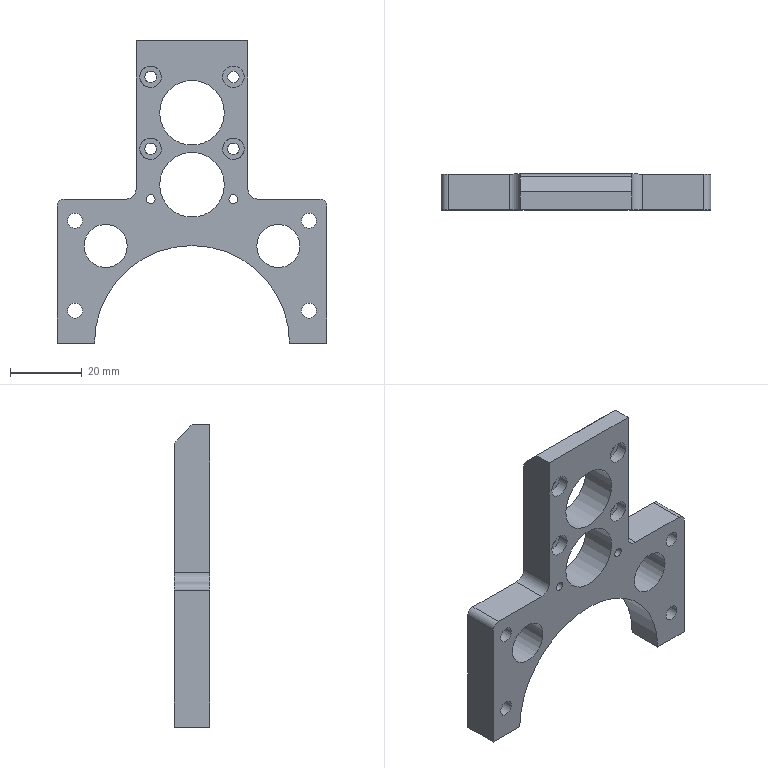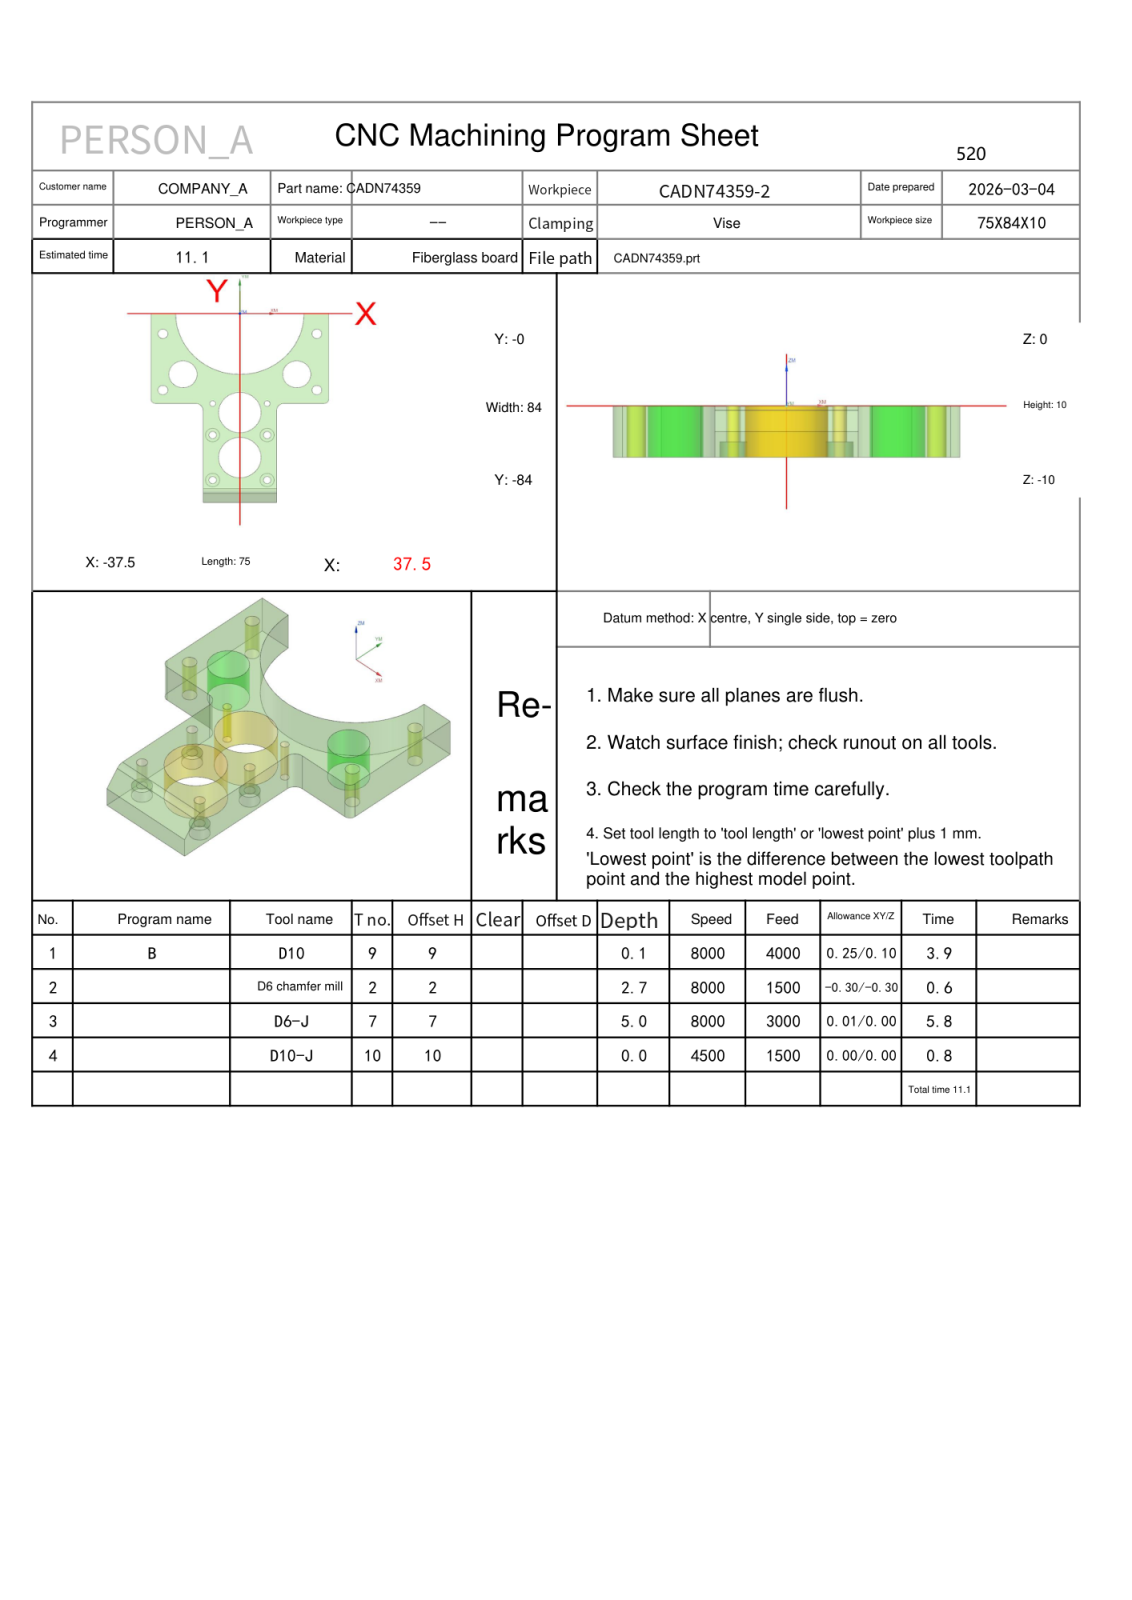NC program | NX | posted by the shop | part box 75 x 10 x 84 mm
Lines 1701 to 1963 of 5701:
N2 T02 M06
(D6 chamfer mill  D=6. R=0. H=02 ce=0.00 di=0.10)
G00 G90 G54 X-11.5 Y-40. M03 S8000
G43 H02 Z50.
M08
G98 G81 X-11.5 Y-40. Z-1.75 R3. F1000.
X11.5
G80
G00 Z50.
G00 G90 X-11.5 Y-74. M03 S8000
Z50.
G98 G81 X-11.5 Y-74. Z-1.9 R3. F1000.
Y-54.
X11.5
Y-74.
G80
G00 Z50.
G00 G90 X32.5 Y-34. M03 S8000
Z50.
G98 G81 X32.5 Y-34. Z-2.7 R3. F1000.
Y-9.
X-32.5
Y-34.
G80
G00 Z50.
G00 G90 X-21. Y-24.7 M03 S8000
Z50.
Z-.5
G01 Z-1. F1200.
G03 X-24. Y-21.7 I-3. J0.0
X-29.3 Y-27. I0.0 J-5.3
X-24. Y-32.3 I5.3 J0.0
X-18.7 Y-27. I0.0 J5.3
X-24. Y-21.7 I-5.3 J0.0
X-27. Y-24.7 I0.0 J-3.
G01 Z-.5
G00 Z50.
X27.
Z-.5
G01 Z-1.
G03 X24. Y-21.7 I-3. J0.0
X18.7 Y-27. I0.0 J-5.3
X24. Y-32.3 I5.3 J0.0
X29.3 Y-27. I0.0 J5.3
X24. Y-21.7 I-5.3 J0.0
X21. Y-24.7 I0.0 J-3.
G01 Z-.5
G00 Z50.
G00 G90 X-16.727 Y-78.143 M03 S6500
Z50.
Z.145
G01 Z-1.2 F1500.
G03 X-16.527 Y-77.857 I-1.532 J1.286
G01 X-16.497 Y-77.812
X-16.5 Y-77.757
Y-43.
G03 X-18.5 Y-41. I-2. J0.0
G01 X-35.5
G02 X-38.5 Y-38. I0.0 J3.
G01 Y0.0
G02 X-37.5 Y1. I1. J0.0
G01 X-27.1
G02 X-26.1 Y0.0 I0.0 J-1.
G03 X0.0 Y-26.1 I26.1 J0.0
X26.1 Y0.0 I0.0 J26.1
G02 X27.1 Y1. I1. J0.0
G01 X37.5
G02 X38.5 Y0.0 I0.0 J-1.
G01 Y-38.
G02 X35.5 Y-41. I-3. J0.0
G01 X18.5
G03 X16.5 Y-43. I0.0 J-2.
G01 Y-77.757
X16.497 Y-77.812
X16.527 Y-77.857
G03 X16.727 Y-78.143 I1.732 J1.
G01 Z.145
G00 Z2.55
X11.919 Y-73.556
Z.417
G01 Z-1.2
G03 X11.603 Y-73.409 I-1. J-1.732
G01 X11.553 Y-73.388
X11.5 Y-73.4
G03 X10.9 Y-74. I0.0 J-.6
X11.5 Y-74.6 I.6 J0.0
X12.1 Y-74. I0.0 J.6
X11.5 Y-73.4 I-.6 J0.0
G01 X11.447 Y-73.388
X11.397 Y-73.409
G03 X11.081 Y-73.556 I.684 J-1.879
G01 Z.417
G00 Z10.
X.396 Y-56.208
Z.209
G01 Z-1.2
G03 X.101 Y-56.022 I-1.211 J-1.592
G01 X.054 Y-55.995
X0.0 Y-56.
G03 X-8. Y-64. I0.0 J-8.
X0.0 Y-72. I8. J0.0
X8. Y-64. I0.0 J8.
X0.0 Y-56. I-8. J0.0
G01 X-.054 Y-55.995
X-.101 Y-56.022
G03 X-.396 Y-56.208 I.916 J-1.778
G01 Z.208
G00 Z10.
X-11.919 Y-74.444
Z.417
G01 Z-1.2
G03 X-11.603 Y-74.591 I1. J1.732
G01 X-11.553 Y-74.612
X-11.5 Y-74.6
G03 X-10.9 Y-74. I0.0 J.6
X-11.5 Y-73.4 I-.6 J0.0
X-12.1 Y-74. I0.0 J-.6
X-11.5 Y-74.6 I.6 J0.0
G01 X-11.447 Y-74.612
X-11.397 Y-74.591
G03 X-11.081 Y-74.444 I-.684 J1.879
G01 Z.417
G00 Z10.
X-11.919 Y-54.444
Z.417
G01 Z-1.2
G03 X-11.603 Y-54.591 I1. J1.732
G01 X-11.553 Y-54.612
X-11.5 Y-54.6
G03 X-10.9 Y-54. I0.0 J.6
X-11.5 Y-53.4 I-.6 J0.0
X-12.1 Y-54. I0.0 J-.6
X-11.5 Y-54.6 I.6 J0.0
G01 X-11.447 Y-54.612
X-11.397 Y-54.591
G03 X-11.081 Y-54.444 I-.684 J1.879
G01 Z.417
G00 Z10.
X-32.912 Y-34.926
Z.321
G01 Z-1.2
G03 X-32.603 Y-35.086 I1.075 J1.687
G01 X-32.554 Y-35.11
X-32.5 Y-35.1
G03 X-31.4 Y-34. I0.0 J1.1
X-32.5 Y-32.9 I-1.1 J0.0
X-33.6 Y-34. I0.0 J-1.1
X-32.5 Y-35.1 I1.1 J0.0
G01 X-32.446 Y-35.11
X-32.397 Y-35.086
G03 X-32.088 Y-34.926 I-.765 J1.848
G01 Z.317
G00 Z10.
X-32.912 Y-9.926
Z.321
G01 Z-1.2
G03 X-32.603 Y-10.086 I1.075 J1.687
G01 X-32.554 Y-10.11
X-32.5 Y-10.1
G03 X-31.4 Y-9. I0.0 J1.1
X-32.5 Y-7.9 I-1.1 J0.0
X-33.6 Y-9. I0.0 J-1.1
X-32.5 Y-10.1 I1.1 J0.0
G01 X-32.446 Y-10.11
X-32.397 Y-10.086
G03 X-32.088 Y-9.926 I-.765 J1.848
G01 Z.317
G00 Z10.
X-23.602 Y-22.204
Z.221
G01 Z-1.2
G03 X-23.899 Y-22.021 I-1.194 J-1.604
G01 X-23.946 Y-21.994
X-24. Y-22.
G03 X-29. Y-27. I0.0 J-5.
X-24. Y-32. I5. J0.0
X-19. Y-27. I0.0 J5.
X-24. Y-22. I-5. J0.0
G01 X-24.054 Y-21.994
X-24.101 Y-22.021
G03 X-24.398 Y-22.204 I.898 J-1.787
G01 Z.214
G00 Z10.
X.396 Y-36.208
Z.209
G01 Z-1.2
G03 X.101 Y-36.022 I-1.211 J-1.592
G01 X.054 Y-35.995
X0.0 Y-36.
G03 X-8. Y-44. I0.0 J-8.
X0.0 Y-52. I8. J0.0
X8. Y-44. I0.0 J8.
X0.0 Y-36. I-8. J0.0
G01 X-.054 Y-35.995
X-.101 Y-36.022
G03 X-.396 Y-36.208 I.916 J-1.778
G01 Z.208
G00 Z10.
X11.919 Y-53.556
Z.417
G01 Z-1.2
G03 X11.603 Y-53.409 I-1. J-1.732
G01 X11.553 Y-53.388
X11.5 Y-53.4
G03 X10.9 Y-54. I0.0 J-.6
X11.5 Y-54.6 I.6 J0.0
X12.1 Y-54. I0.0 J.6
X11.5 Y-53.4 I-.6 J0.0
G01 X11.447 Y-53.388
X11.397 Y-53.409
G03 X11.081 Y-53.556 I.684 J-1.879
G01 Z.417
G00 Z10.
X32.088 Y-34.926
Z.321
G01 Z-1.2
G03 X32.397 Y-35.086 I1.075 J1.687
G01 X32.446 Y-35.11
X32.5 Y-35.1
G03 X33.6 Y-34. I0.0 J1.1
X32.5 Y-32.9 I-1.1 J0.0
X31.4 Y-34. I0.0 J-1.1
X32.5 Y-35.1 I1.1 J0.0
G01 X32.554 Y-35.11
X32.603 Y-35.086
G03 X32.912 Y-34.926 I-.765 J1.848
G01 Z.317
G00 Z10.
X24.398 Y-22.204
Z.221
G01 Z-1.2
G03 X24.101 Y-22.021 I-1.194 J-1.604
G01 X24.054 Y-21.994
X24. Y-22.
G03 X19. Y-27. I0.0 J-5.
X24. Y-32. I5. J0.0
X29. Y-27. I0.0 J5.
X24. Y-22. I-5. J0.0
G01 X23.946 Y-21.994
X23.899 Y-22.021
G03 X23.602 Y-22.204 I.898 J-1.787
G01 Z.214
G00 Z10.
X32.088 Y-9.926
Z.321
G01 Z-1.2
G03 X32.397 Y-10.086 I1.075 J1.687
G01 X32.446 Y-10.11
X32.5 Y-10.1
G03 X33.6 Y-9. I0.0 J1.1
X32.5 Y-7.9 I-1.1 J0.0
X31.4 Y-9. I0.0 J-1.1
X32.5 Y-10.1 I1.1 J0.0
G01 X32.554 Y-10.11
X32.603 Y-10.086
G03 X32.912 Y-9.926 I-.765 J1.848
G01 Z.317
G00 Z50.
G91 G28 Z0.0
M05
M09
G91 G28 Z0.0
M01